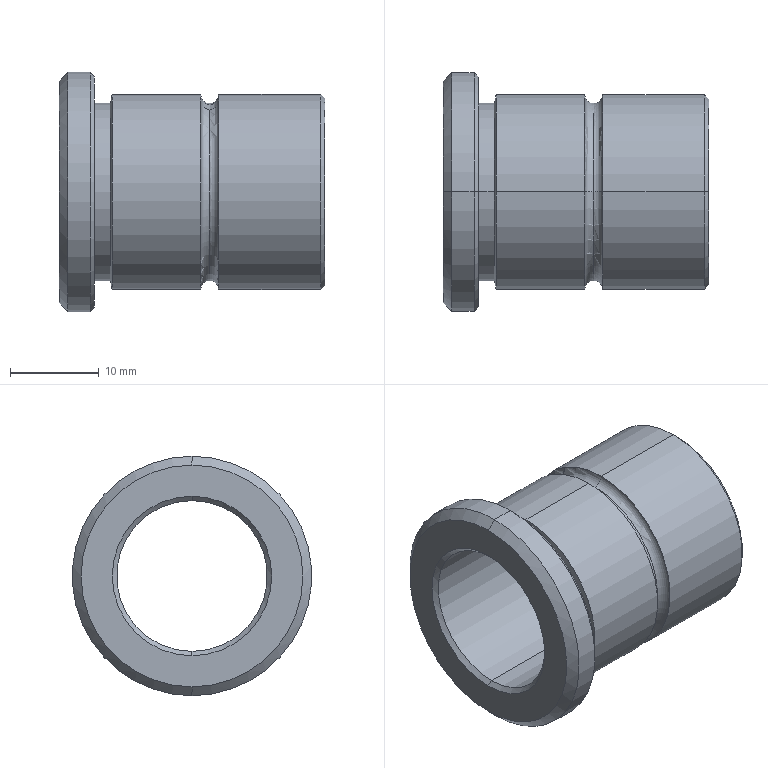Part | SolidWorks | features Chamfer 2, RefAxis 1, RevCut 1, Revolution 1 | 1 solid | 29 faces | box 30 x 27 x 27 mm | volume 5060 mm3 | cone 12 | cylinder 10 | torus 4 | plane 3 | commonest cylinder face diameters 22 x4 17 x2 20 x2 27 x2
STEP:
#1=CARTESIAN_POINT('',(18.,0.,-11.));
#2=VERTEX_POINT('',#1);
#3=CARTESIAN_POINT('',(17.,0.,-10.));
#4=VERTEX_POINT('',#3);
#5=CARTESIAN_POINT('',(17.,0.,-11.));
#6=DIRECTION('',(0.,-1.,0.));
#7=DIRECTION('',(0.,0.,-1.));
#8=AXIS2_PLACEMENT_3D('',#5,#6,#7);
#9=CIRCLE('',#8,1.);
#10=EDGE_CURVE('',#2,#4,#9,.T.);
#11=ORIENTED_EDGE('',*,*,#10,.T.);
#12=CARTESIAN_POINT('',(17.,0.,10.));
#13=VERTEX_POINT('',#12);
#14=CARTESIAN_POINT('',(17.,0.,0.));
#15=DIRECTION('',(1.,0.,0.));
#16=DIRECTION('',(0.,0.,-1.));
#17=AXIS2_PLACEMENT_3D('',#14,#15,#16);
#18=CIRCLE('',#17,10.);
#19=EDGE_CURVE('',#4,#13,#18,.T.);
#20=ORIENTED_EDGE('',*,*,#19,.T.);
#21=CARTESIAN_POINT('',(18.,0.,11.));
#22=VERTEX_POINT('',#21);
#23=CARTESIAN_POINT('',(17.,0.,11.));
#24=DIRECTION('',(0.,1.,0.));
#25=DIRECTION('',(0.,0.,1.));
#26=AXIS2_PLACEMENT_3D('',#23,#24,#25);
#27=CIRCLE('',#26,1.);
#28=EDGE_CURVE('',#22,#13,#27,.T.);
#29=ORIENTED_EDGE('',*,*,#28,.F.);
#30=CARTESIAN_POINT('',(18.,0.,0.));
#31=DIRECTION('',(1.,0.,0.));
#32=DIRECTION('',(0.,0.,1.));
#33=AXIS2_PLACEMENT_3D('',#30,#31,#32);
#34=CIRCLE('',#33,11.);
#35=EDGE_CURVE('',#2,#22,#34,.T.);
#36=ORIENTED_EDGE('',*,*,#35,.F.);
#37=EDGE_LOOP('',(#11,#20,#29,#36));
#38=FACE_OUTER_BOUND('',#37,.T.);
#39=CARTESIAN_POINT('',(17.,0.,0.));
#40=DIRECTION('',(1.,0.,0.));
#41=DIRECTION('',(0.,0.,-1.));
#42=AXIS2_PLACEMENT_3D('',#39,#40,#41);
#43=TOROIDAL_SURFACE('',#42,11.,1.);
#44=ADVANCED_FACE('',(#38),#43,.F.);
#45=ORIENTED_EDGE('',*,*,#28,.T.);
#46=CARTESIAN_POINT('',(17.,0.,0.));
#47=DIRECTION('',(1.,0.,0.));
#48=DIRECTION('',(0.,0.,-1.));
#49=AXIS2_PLACEMENT_3D('',#46,#47,#48);
#50=CIRCLE('',#49,10.);
#51=EDGE_CURVE('',#13,#4,#50,.T.);
#52=ORIENTED_EDGE('',*,*,#51,.T.);
#53=ORIENTED_EDGE('',*,*,#10,.F.);
#54=CARTESIAN_POINT('',(18.,0.,0.));
#55=DIRECTION('',(1.,0.,0.));
#56=DIRECTION('',(0.,0.,1.));
#57=AXIS2_PLACEMENT_3D('',#54,#55,#56);
#58=CIRCLE('',#57,11.);
#59=EDGE_CURVE('',#22,#2,#58,.T.);
#60=ORIENTED_EDGE('',*,*,#59,.F.);
#61=EDGE_LOOP('',(#45,#52,#53,#60));
#62=FACE_OUTER_BOUND('',#61,.T.);
#63=CARTESIAN_POINT('',(17.,0.,0.));
#64=DIRECTION('',(1.,0.,0.));
#65=DIRECTION('',(0.,0.,-1.));
#66=AXIS2_PLACEMENT_3D('',#63,#64,#65);
#67=TOROIDAL_SURFACE('',#66,11.,1.);
#68=ADVANCED_FACE('',(#62),#67,.F.);
#69=CARTESIAN_POINT('',(5.8,0.,-10.));
#70=VERTEX_POINT('',#69);
#71=CARTESIAN_POINT('',(5.8,0.,10.));
#72=VERTEX_POINT('',#71);
#73=CARTESIAN_POINT('',(5.8,0.,0.));
#74=DIRECTION('',(1.,0.,0.));
#75=DIRECTION('',(0.,0.,-1.));
#76=AXIS2_PLACEMENT_3D('',#73,#74,#75);
#77=CIRCLE('',#76,10.);
#78=EDGE_CURVE('',#70,#72,#77,.T.);
#79=ORIENTED_EDGE('',*,*,#78,.T.);
#80=CARTESIAN_POINT('',(6.,0.,11.));
#81=VERTEX_POINT('',#80);
#82=CARTESIAN_POINT('',(5.8,0.,10.));
#83=DIRECTION('',(0.1961,0.,0.9806));
#84=VECTOR('',#83,1000.);
#85=LINE('',#82,#84);
#86=EDGE_CURVE('',#72,#81,#85,.T.);
#87=ORIENTED_EDGE('',*,*,#86,.T.);
#88=CARTESIAN_POINT('',(6.,0.,-11.));
#89=VERTEX_POINT('',#88);
#90=CARTESIAN_POINT('',(6.,0.,0.));
#91=DIRECTION('',(1.,0.,0.));
#92=DIRECTION('',(0.,0.,-1.));
#93=AXIS2_PLACEMENT_3D('',#90,#91,#92);
#94=CIRCLE('',#93,11.);
#95=EDGE_CURVE('',#89,#81,#94,.T.);
#96=ORIENTED_EDGE('',*,*,#95,.F.);
#97=CARTESIAN_POINT('',(5.8,0.,-10.));
#98=DIRECTION('',(0.1961,0.,-0.9806));
#99=VECTOR('',#98,1000.);
#100=LINE('',#97,#99);
#101=EDGE_CURVE('',#70,#89,#100,.T.);
#102=ORIENTED_EDGE('',*,*,#101,.F.);
#103=EDGE_LOOP('',(#79,#87,#96,#102));
#104=FACE_OUTER_BOUND('',#103,.T.);
#105=CARTESIAN_POINT('',(5.8,0.,0.));
#106=DIRECTION('',(1.,0.,0.));
#107=DIRECTION('',(0.,0.,-1.));
#108=AXIS2_PLACEMENT_3D('',#105,#106,#107);
#109=CONICAL_SURFACE('',#108,10.,1.373);
#110=ADVANCED_FACE('',(#104),#109,.T.);
#111=CARTESIAN_POINT('',(4.,0.,-10.));
#112=VERTEX_POINT('',#111);
#113=CARTESIAN_POINT('',(4.,0.,10.));
#114=VERTEX_POINT('',#113);
#115=CARTESIAN_POINT('',(4.,0.,0.));
#116=DIRECTION('',(1.,0.,0.));
#117=DIRECTION('',(0.,0.,-1.));
#118=AXIS2_PLACEMENT_3D('',#115,#116,#117);
#119=CIRCLE('',#118,10.);
#120=EDGE_CURVE('',#112,#114,#119,.T.);
#121=ORIENTED_EDGE('',*,*,#120,.T.);
#122=CARTESIAN_POINT('',(29.5,0.,10.));
#123=DIRECTION('',(1.,0.,0.));
#124=VECTOR('',#123,1000.);
#125=LINE('',#122,#124);
#126=EDGE_CURVE('',#114,#72,#125,.T.);
#127=ORIENTED_EDGE('',*,*,#126,.T.);
#128=ORIENTED_EDGE('',*,*,#78,.F.);
#129=CARTESIAN_POINT('',(29.5,0.,-10.));
#130=DIRECTION('',(1.,0.,0.));
#131=VECTOR('',#130,1000.);
#132=LINE('',#129,#131);
#133=EDGE_CURVE('',#112,#70,#132,.T.);
#134=ORIENTED_EDGE('',*,*,#133,.F.);
#135=EDGE_LOOP('',(#121,#127,#128,#134));
#136=FACE_OUTER_BOUND('',#135,.T.);
#137=CARTESIAN_POINT('',(29.5,0.,0.));
#138=DIRECTION('',(1.,0.,0.));
#139=DIRECTION('',(0.,0.,-1.));
#140=AXIS2_PLACEMENT_3D('',#137,#138,#139);
#141=CYLINDRICAL_SURFACE('',#140,10.);
#142=ADVANCED_FACE('',(#136),#141,.T.);
#143=ORIENTED_EDGE('',*,*,#51,.F.);
#144=CARTESIAN_POINT('',(16.,0.,11.));
#145=VERTEX_POINT('',#144);
#146=CARTESIAN_POINT('',(17.,0.,11.));
#147=DIRECTION('',(0.,1.,0.));
#148=DIRECTION('',(0.,0.,1.));
#149=AXIS2_PLACEMENT_3D('',#146,#147,#148);
#150=CIRCLE('',#149,1.);
#151=EDGE_CURVE('',#13,#145,#150,.T.);
#152=ORIENTED_EDGE('',*,*,#151,.T.);
#153=CARTESIAN_POINT('',(16.,0.,-11.));
#154=VERTEX_POINT('',#153);
#155=CARTESIAN_POINT('',(16.,0.,0.));
#156=DIRECTION('',(-1.,0.,0.));
#157=DIRECTION('',(0.,0.,-1.));
#158=AXIS2_PLACEMENT_3D('',#155,#156,#157);
#159=CIRCLE('',#158,11.);
#160=EDGE_CURVE('',#154,#145,#159,.T.);
#161=ORIENTED_EDGE('',*,*,#160,.F.);
#162=CARTESIAN_POINT('',(17.,0.,-11.));
#163=DIRECTION('',(0.,-1.,0.));
#164=DIRECTION('',(0.,0.,-1.));
#165=AXIS2_PLACEMENT_3D('',#162,#163,#164);
#166=CIRCLE('',#165,1.);
#167=EDGE_CURVE('',#4,#154,#166,.T.);
#168=ORIENTED_EDGE('',*,*,#167,.F.);
#169=EDGE_LOOP('',(#143,#152,#161,#168));
#170=FACE_OUTER_BOUND('',#169,.T.);
#171=CARTESIAN_POINT('',(17.,0.,0.));
#172=DIRECTION('',(1.,0.,0.));
#173=DIRECTION('',(0.,0.,-1.));
#174=AXIS2_PLACEMENT_3D('',#171,#172,#173);
#175=TOROIDAL_SURFACE('',#174,11.,1.);
#176=ADVANCED_FACE('',(#170),#175,.F.);
#177=CARTESIAN_POINT('',(30.,0.,-10.5));
#178=VERTEX_POINT('',#177);
#179=CARTESIAN_POINT('',(30.,0.,10.5));
#180=VERTEX_POINT('',#179);
#181=CARTESIAN_POINT('',(30.,0.,0.));
#182=DIRECTION('',(1.,0.,0.));
#183=DIRECTION('',(0.,0.,1.));
#184=AXIS2_PLACEMENT_3D('',#181,#182,#183);
#185=CIRCLE('',#184,10.5);
#186=EDGE_CURVE('',#178,#180,#185,.T.);
#187=ORIENTED_EDGE('',*,*,#186,.F.);
#188=CARTESIAN_POINT('',(29.5,0.,-11.));
#189=VERTEX_POINT('',#188);
#190=CARTESIAN_POINT('',(29.5,0.,-11.));
#191=DIRECTION('',(-0.7071,0.,-0.7071));
#192=VECTOR('',#191,1000.);
#193=LINE('',#190,#192);
#194=EDGE_CURVE('',#178,#189,#193,.T.);
#195=ORIENTED_EDGE('',*,*,#194,.T.);
#196=CARTESIAN_POINT('',(29.5,0.,11.));
#197=VERTEX_POINT('',#196);
#198=CARTESIAN_POINT('',(29.5,0.,0.));
#199=DIRECTION('',(-1.,0.,0.));
#200=DIRECTION('',(0.,0.,1.));
#201=AXIS2_PLACEMENT_3D('',#198,#199,#200);
#202=CIRCLE('',#201,11.);
#203=EDGE_CURVE('',#197,#189,#202,.T.);
#204=ORIENTED_EDGE('',*,*,#203,.F.);
#205=CARTESIAN_POINT('',(29.5,0.,11.));
#206=DIRECTION('',(-0.7071,0.,0.7071));
#207=VECTOR('',#206,1000.);
#208=LINE('',#205,#207);
#209=EDGE_CURVE('',#180,#197,#208,.T.);
#210=ORIENTED_EDGE('',*,*,#209,.F.);
#211=EDGE_LOOP('',(#187,#195,#204,#210));
#212=FACE_OUTER_BOUND('',#211,.T.);
#213=CARTESIAN_POINT('',(29.5,0.,0.));
#214=DIRECTION('',(-1.,0.,0.));
#215=DIRECTION('',(0.,0.,1.));
#216=AXIS2_PLACEMENT_3D('',#213,#214,#215);
#217=CONICAL_SURFACE('',#216,11.,0.7854);
#218=ADVANCED_FACE('',(#212),#217,.T.);
#219=CARTESIAN_POINT('',(29.5,0.,8.5));
#220=VERTEX_POINT('',#219);
#221=CARTESIAN_POINT('',(29.5,0.,-8.5));
#222=VERTEX_POINT('',#221);
#223=CARTESIAN_POINT('',(29.5,0.,0.));
#224=DIRECTION('',(1.,0.,0.));
#225=DIRECTION('',(0.,0.,1.));
#226=AXIS2_PLACEMENT_3D('',#223,#224,#225);
#227=CIRCLE('',#226,8.5);
#228=EDGE_CURVE('',#220,#222,#227,.T.);
#229=ORIENTED_EDGE('',*,*,#228,.F.);
#230=CARTESIAN_POINT('',(30.,0.,9.));
#231=VERTEX_POINT('',#230);
#232=CARTESIAN_POINT('',(30.,0.,9.));
#233=DIRECTION('',(0.7071,0.,0.7071));
#234=VECTOR('',#233,1000.);
#235=LINE('',#232,#234);
#236=EDGE_CURVE('',#220,#231,#235,.T.);
#237=ORIENTED_EDGE('',*,*,#236,.T.);
#238=CARTESIAN_POINT('',(30.,0.,-9.));
#239=VERTEX_POINT('',#238);
#240=CARTESIAN_POINT('',(30.,0.,0.));
#241=DIRECTION('',(-1.,0.,0.));
#242=DIRECTION('',(0.,0.,1.));
#243=AXIS2_PLACEMENT_3D('',#240,#241,#242);
#244=CIRCLE('',#243,9.);
#245=EDGE_CURVE('',#239,#231,#244,.T.);
#246=ORIENTED_EDGE('',*,*,#245,.F.);
#247=CARTESIAN_POINT('',(30.,0.,-9.));
#248=DIRECTION('',(0.7071,0.,-0.7071));
#249=VECTOR('',#248,1000.);
#250=LINE('',#247,#249);
#251=EDGE_CURVE('',#222,#239,#250,.T.);
#252=ORIENTED_EDGE('',*,*,#251,.F.);
#253=EDGE_LOOP('',(#229,#237,#246,#252));
#254=FACE_OUTER_BOUND('',#253,.T.);
#255=CARTESIAN_POINT('',(30.,0.,0.));
#256=DIRECTION('',(1.,0.,0.));
#257=DIRECTION('',(0.,0.,-1.));
#258=AXIS2_PLACEMENT_3D('',#255,#256,#257);
#259=CONICAL_SURFACE('',#258,9.,0.7854);
#260=ADVANCED_FACE('',(#254),#259,.F.);
#261=CARTESIAN_POINT('',(0.5,0.,-8.5));
#262=VERTEX_POINT('',#261);
#263=CARTESIAN_POINT('',(0.5,0.,8.5));
#264=VERTEX_POINT('',#263);
#265=CARTESIAN_POINT('',(0.5,0.,0.));
#266=DIRECTION('',(-1.,0.,0.));
#267=DIRECTION('',(0.,0.,-1.));
#268=AXIS2_PLACEMENT_3D('',#265,#266,#267);
#269=CIRCLE('',#268,8.5);
#270=EDGE_CURVE('',#262,#264,#269,.T.);
#271=ORIENTED_EDGE('',*,*,#270,.F.);
#272=CARTESIAN_POINT('',(0.,0.,-9.));
#273=VERTEX_POINT('',#272);
#274=CARTESIAN_POINT('',(0.5,0.,-8.5));
#275=DIRECTION('',(-0.7071,0.,-0.7071));
#276=VECTOR('',#275,1000.);
#277=LINE('',#274,#276);
#278=EDGE_CURVE('',#262,#273,#277,.T.);
#279=ORIENTED_EDGE('',*,*,#278,.T.);
#280=CARTESIAN_POINT('',(0.,0.,9.));
#281=VERTEX_POINT('',#280);
#282=CARTESIAN_POINT('',(0.,0.,0.));
#283=DIRECTION('',(1.,0.,0.));
#284=DIRECTION('',(0.,0.,-1.));
#285=AXIS2_PLACEMENT_3D('',#282,#283,#284);
#286=CIRCLE('',#285,9.);
#287=EDGE_CURVE('',#281,#273,#286,.T.);
#288=ORIENTED_EDGE('',*,*,#287,.F.);
#289=CARTESIAN_POINT('',(0.5,0.,8.5));
#290=DIRECTION('',(-0.7071,0.,0.7071));
#291=VECTOR('',#290,1000.);
#292=LINE('',#289,#291);
#293=EDGE_CURVE('',#264,#281,#292,.T.);
#294=ORIENTED_EDGE('',*,*,#293,.F.);
#295=EDGE_LOOP('',(#271,#279,#288,#294));
#296=FACE_OUTER_BOUND('',#295,.T.);
#297=CARTESIAN_POINT('',(0.5,0.,0.));
#298=DIRECTION('',(-1.,0.,0.));
#299=DIRECTION('',(0.,0.,1.));
#300=AXIS2_PLACEMENT_3D('',#297,#298,#299);
#301=CONICAL_SURFACE('',#300,8.5,0.7854);
#302=ADVANCED_FACE('',(#296),#301,.F.);
#303=CARTESIAN_POINT('',(4.,0.,-13.));
#304=VERTEX_POINT('',#303);
#305=CARTESIAN_POINT('',(4.,0.,13.));
#306=VERTEX_POINT('',#305);
#307=CARTESIAN_POINT('',(4.,0.,0.));
#308=DIRECTION('',(1.,0.,0.));
#309=DIRECTION('',(0.,0.,1.));
#310=AXIS2_PLACEMENT_3D('',#307,#308,#309);
#311=CIRCLE('',#310,13.);
#312=EDGE_CURVE('',#304,#306,#311,.T.);
#313=ORIENTED_EDGE('',*,*,#312,.F.);
#314=CARTESIAN_POINT('',(3.5,0.,-13.5));
#315=VERTEX_POINT('',#314);
#316=CARTESIAN_POINT('',(3.5,0.,-13.5));
#317=DIRECTION('',(-0.7071,0.,-0.7071));
#318=VECTOR('',#317,1000.);
#319=LINE('',#316,#318);
#320=EDGE_CURVE('',#304,#315,#319,.T.);
#321=ORIENTED_EDGE('',*,*,#320,.T.);
#322=CARTESIAN_POINT('',(3.5,0.,13.5));
#323=VERTEX_POINT('',#322);
#324=CARTESIAN_POINT('',(3.5,0.,0.));
#325=DIRECTION('',(-1.,0.,0.));
#326=DIRECTION('',(0.,0.,1.));
#327=AXIS2_PLACEMENT_3D('',#324,#325,#326);
#328=CIRCLE('',#327,13.5);
#329=EDGE_CURVE('',#323,#315,#328,.T.);
#330=ORIENTED_EDGE('',*,*,#329,.F.);
#331=CARTESIAN_POINT('',(3.5,0.,13.5));
#332=DIRECTION('',(-0.7071,0.,0.7071));
#333=VECTOR('',#332,1000.);
#334=LINE('',#331,#333);
#335=EDGE_CURVE('',#306,#323,#334,.T.);
#336=ORIENTED_EDGE('',*,*,#335,.F.);
#337=EDGE_LOOP('',(#313,#321,#330,#336));
#338=FACE_OUTER_BOUND('',#337,.T.);
#339=CARTESIAN_POINT('',(3.5,0.,0.));
#340=DIRECTION('',(-1.,0.,0.));
#341=DIRECTION('',(0.,0.,1.));
#342=AXIS2_PLACEMENT_3D('',#339,#340,#341);
#343=CONICAL_SURFACE('',#342,13.5,0.7854);
#344=ADVANCED_FACE('',(#338),#343,.T.);
#345=CARTESIAN_POINT('',(0.,0.,12.5));
#346=VERTEX_POINT('',#345);
#347=CARTESIAN_POINT('',(0.,0.,-12.5));
#348=VERTEX_POINT('',#347);
#349=CARTESIAN_POINT('',(0.,0.,0.));
#350=DIRECTION('',(-1.,0.,0.));
#351=DIRECTION('',(0.,0.,-1.));
#352=AXIS2_PLACEMENT_3D('',#349,#350,#351);
#353=CIRCLE('',#352,12.5);
#354=EDGE_CURVE('',#346,#348,#353,.T.);
#355=ORIENTED_EDGE('',*,*,#354,.F.);
#356=CARTESIAN_POINT('',(1.,0.,13.5));
#357=VERTEX_POINT('',#356);
#358=CARTESIAN_POINT('',(0.,0.,12.5));
#359=DIRECTION('',(0.7071,0.,0.7071));
#360=VECTOR('',#359,1000.);
#361=LINE('',#358,#360);
#362=EDGE_CURVE('',#346,#357,#361,.T.);
#363=ORIENTED_EDGE('',*,*,#362,.T.);
#364=CARTESIAN_POINT('',(1.,0.,-13.5));
#365=VERTEX_POINT('',#364);
#366=CARTESIAN_POINT('',(1.,0.,0.));
#367=DIRECTION('',(1.,0.,0.));
#368=DIRECTION('',(0.,0.,-1.));
#369=AXIS2_PLACEMENT_3D('',#366,#367,#368);
#370=CIRCLE('',#369,13.5);
#371=EDGE_CURVE('',#365,#357,#370,.T.);
#372=ORIENTED_EDGE('',*,*,#371,.F.);
#373=CARTESIAN_POINT('',(0.,0.,-12.5));
#374=DIRECTION('',(0.7071,0.,-0.7071));
#375=VECTOR('',#374,1000.);
#376=LINE('',#373,#375);
#377=EDGE_CURVE('',#348,#365,#376,.T.);
#378=ORIENTED_EDGE('',*,*,#377,.F.);
#379=EDGE_LOOP('',(#355,#363,#372,#378));
#380=FACE_OUTER_BOUND('',#379,.T.);
#381=CARTESIAN_POINT('',(0.,0.,0.));
#382=DIRECTION('',(1.,0.,0.));
#383=DIRECTION('',(0.,0.,-1.));
#384=AXIS2_PLACEMENT_3D('',#381,#382,#383);
#385=CONICAL_SURFACE('',#384,12.5,0.7854);
#386=ADVANCED_FACE('',(#380),#385,.T.);
#387=CARTESIAN_POINT('',(16.,0.,0.));
#388=DIRECTION('',(-1.,0.,0.));
#389=DIRECTION('',(0.,0.,-1.));
#390=AXIS2_PLACEMENT_3D('',#387,#388,#389);
#391=CIRCLE('',#390,11.);
#392=EDGE_CURVE('',#145,#154,#391,.T.);
#393=ORIENTED_EDGE('',*,*,#392,.T.);
#394=CARTESIAN_POINT('',(0.,0.,-11.));
#395=DIRECTION('',(-1.,0.,0.));
#396=VECTOR('',#395,1000.);
#397=LINE('',#394,#396);
#398=EDGE_CURVE('',#154,#89,#397,.T.);
#399=ORIENTED_EDGE('',*,*,#398,.T.);
#400=ORIENTED_EDGE('',*,*,#95,.T.);
#401=CARTESIAN_POINT('',(0.,0.,11.));
#402=DIRECTION('',(-1.,0.,0.));
#403=VECTOR('',#402,1000.);
#404=LINE('',#401,#403);
#405=EDGE_CURVE('',#145,#81,#404,.T.);
#406=ORIENTED_EDGE('',*,*,#405,.F.);
#407=EDGE_LOOP('',(#393,#399,#400,#406));
#408=FACE_OUTER_BOUND('',#407,.T.);
#409=CARTESIAN_POINT('',(0.,0.,0.));
#410=DIRECTION('',(-1.,0.,0.));
#411=DIRECTION('',(0.,0.,1.));
#412=AXIS2_PLACEMENT_3D('',#409,#410,#411);
#413=CYLINDRICAL_SURFACE('',#412,11.);
#414=ADVANCED_FACE('',(#408),#413,.T.);
#415=ORIENTED_EDGE('',*,*,#329,.T.);
#416=CARTESIAN_POINT('',(0.,0.,-13.5));
#417=DIRECTION('',(-1.,0.,0.));
#418=VECTOR('',#417,1000.);
#419=LINE('',#416,#418);
#420=EDGE_CURVE('',#315,#365,#419,.T.);
#421=ORIENTED_EDGE('',*,*,#420,.T.);
#422=ORIENTED_EDGE('',*,*,#371,.T.);
#423=CARTESIAN_POINT('',(0.,0.,13.5));
#424=DIRECTION('',(-1.,0.,0.));
#425=VECTOR('',#424,1000.);
#426=LINE('',#423,#425);
#427=EDGE_CURVE('',#323,#357,#426,.T.);
#428=ORIENTED_EDGE('',*,*,#427,.F.);
#429=EDGE_LOOP('',(#415,#421,#422,#428));
#430=FACE_OUTER_BOUND('',#429,.T.);
#431=CARTESIAN_POINT('',(0.,0.,0.));
#432=DIRECTION('',(-1.,0.,0.));
#433=DIRECTION('',(0.,0.,1.));
#434=AXIS2_PLACEMENT_3D('',#431,#432,#433);
#435=CYLINDRICAL_SURFACE('',#434,13.5);
#436=ADVANCED_FACE('',(#430),#435,.T.);
#437=ORIENTED_EDGE('',*,*,#228,.T.);
#438=CARTESIAN_POINT('',(0.,0.,-8.5));
#439=DIRECTION('',(-1.,0.,0.));
#440=VECTOR('',#439,1000.);
#441=LINE('',#438,#440);
#442=EDGE_CURVE('',#222,#262,#441,.T.);
#443=ORIENTED_EDGE('',*,*,#442,.T.);
#444=ORIENTED_EDGE('',*,*,#270,.T.);
#445=CARTESIAN_POINT('',(0.,0.,8.5));
#446=DIRECTION('',(-1.,0.,0.));
#447=VECTOR('',#446,1000.);
#448=LINE('',#445,#447);
#449=EDGE_CURVE('',#220,#264,#448,.T.);
#450=ORIENTED_EDGE('',*,*,#449,.F.);
#451=EDGE_LOOP('',(#437,#443,#444,#450));
#452=FACE_OUTER_BOUND('',#451,.T.);
#453=CARTESIAN_POINT('',(0.,0.,0.));
#454=DIRECTION('',(-1.,0.,0.));
#455=DIRECTION('',(0.,0.,1.));
#456=AXIS2_PLACEMENT_3D('',#453,#454,#455);
#457=CYLINDRICAL_SURFACE('',#456,8.5);
#458=ADVANCED_FACE('',(#452),#457,.F.);
#459=ORIENTED_EDGE('',*,*,#203,.T.);
#460=CARTESIAN_POINT('',(0.,0.,-11.));
#461=DIRECTION('',(-1.,0.,0.));
#462=VECTOR('',#461,1000.);
#463=LINE('',#460,#462);
#464=EDGE_CURVE('',#189,#2,#463,.T.);
#465=ORIENTED_EDGE('',*,*,#464,.T.);
#466=ORIENTED_EDGE('',*,*,#35,.T.);
#467=CARTESIAN_POINT('',(0.,0.,11.));
#468=DIRECTION('',(-1.,0.,0.));
#469=VECTOR('',#468,1000.);
#470=LINE('',#467,#469);
#471=EDGE_CURVE('',#197,#22,#470,.T.);
#472=ORIENTED_EDGE('',*,*,#471,.F.);
#473=EDGE_LOOP('',(#459,#465,#466,#472));
#474=FACE_OUTER_BOUND('',#473,.T.);
#475=CARTESIAN_POINT('',(0.,0.,0.));
#476=DIRECTION('',(-1.,0.,0.));
#477=DIRECTION('',(0.,0.,1.));
#478=AXIS2_PLACEMENT_3D('',#475,#476,#477);
#479=CYLINDRICAL_SURFACE('',#478,11.);
#480=ADVANCED_FACE('',(#474),#479,.T.);
#481=ORIENTED_EDGE('',*,*,#464,.F.);
#482=CARTESIAN_POINT('',(29.5,0.,0.));
#483=DIRECTION('',(-1.,0.,0.));
#484=DIRECTION('',(0.,0.,1.));
#485=AXIS2_PLACEMENT_3D('',#482,#483,#484);
#486=CIRCLE('',#485,11.);
#487=EDGE_CURVE('',#189,#197,#486,.T.);
#488=ORIENTED_EDGE('',*,*,#487,.T.);
#489=ORIENTED_EDGE('',*,*,#471,.T.);
#490=ORIENTED_EDGE('',*,*,#59,.T.);
#491=EDGE_LOOP('',(#481,#488,#489,#490));
#492=FACE_OUTER_BOUND('',#491,.T.);
#493=CARTESIAN_POINT('',(0.,0.,0.));
#494=DIRECTION('',(-1.,0.,0.));
#495=DIRECTION('',(0.,0.,1.));
#496=AXIS2_PLACEMENT_3D('',#493,#494,#495);
#497=CYLINDRICAL_SURFACE('',#496,11.);
#498=ADVANCED_FACE('',(#492),#497,.T.);
#499=ORIENTED_EDGE('',*,*,#245,.T.);
#500=CARTESIAN_POINT('',(30.,0.,0.));
#501=DIRECTION('',(-1.,0.,0.));
#502=DIRECTION('',(0.,0.,1.));
#503=AXIS2_PLACEMENT_3D('',#500,#501,#502);
#504=CIRCLE('',#503,9.);
#505=EDGE_CURVE('',#231,#239,#504,.T.);
#506=ORIENTED_EDGE('',*,*,#505,.T.);
#507=EDGE_LOOP('',(#499,#506));
#508=FACE_BOUND('',#507,.T.);
#509=CARTESIAN_POINT('',(30.,0.,0.));
#510=DIRECTION('',(1.,0.,0.));
#511=DIRECTION('',(0.,0.,1.));
#512=AXIS2_PLACEMENT_3D('',#509,#510,#511);
#513=CIRCLE('',#512,10.5);
#514=EDGE_CURVE('',#180,#178,#513,.T.);
#515=ORIENTED_EDGE('',*,*,#514,.T.);
#516=ORIENTED_EDGE('',*,*,#186,.T.);
#517=EDGE_LOOP('',(#515,#516));
#518=FACE_OUTER_BOUND('',#517,.T.);
#519=CARTESIAN_POINT('',(30.,11.,0.));
#520=DIRECTION('',(-1.,0.,0.));
#521=DIRECTION('',(0.,0.,1.));
#522=AXIS2_PLACEMENT_3D('',#519,#520,#521);
#523=PLANE('',#522);
#524=ADVANCED_FACE('',(#508,#518),#523,.F.);
#525=ORIENTED_EDGE('',*,*,#442,.F.);
#526=CARTESIAN_POINT('',(29.5,0.,0.));
#527=DIRECTION('',(1.,0.,0.));
#528=DIRECTION('',(0.,0.,1.));
#529=AXIS2_PLACEMENT_3D('',#526,#527,#528);
#530=CIRCLE('',#529,8.5);
#531=EDGE_CURVE('',#222,#220,#530,.T.);
#532=ORIENTED_EDGE('',*,*,#531,.T.);
#533=ORIENTED_EDGE('',*,*,#449,.T.);
#534=CARTESIAN_POINT('',(0.5,0.,0.));
#535=DIRECTION('',(-1.,0.,0.));
#536=DIRECTION('',(0.,0.,-1.));
#537=AXIS2_PLACEMENT_3D('',#534,#535,#536);
#538=CIRCLE('',#537,8.5);
#539=EDGE_CURVE('',#264,#262,#538,.T.);
#540=ORIENTED_EDGE('',*,*,#539,.T.);
#541=EDGE_LOOP('',(#525,#532,#533,#540));
#542=FACE_OUTER_BOUND('',#541,.T.);
#543=CARTESIAN_POINT('',(0.,0.,0.));
#544=DIRECTION('',(-1.,0.,0.));
#545=DIRECTION('',(0.,0.,1.));
#546=AXIS2_PLACEMENT_3D('',#543,#544,#545);
#547=CYLINDRICAL_SURFACE('',#546,8.5);
#548=ADVANCED_FACE('',(#542),#547,.F.);
#549=ORIENTED_EDGE('',*,*,#287,.T.);
#550=CARTESIAN_POINT('',(0.,0.,0.));
#551=DIRECTION('',(1.,0.,0.));
#552=DIRECTION('',(0.,0.,-1.));
#553=AXIS2_PLACEMENT_3D('',#550,#551,#552);
#554=CIRCLE('',#553,9.);
#555=EDGE_CURVE('',#273,#281,#554,.T.);
#556=ORIENTED_EDGE('',*,*,#555,.T.);
#557=EDGE_LOOP('',(#549,#556));
#558=FACE_BOUND('',#557,.T.);
#559=CARTESIAN_POINT('',(0.,0.,0.));
#560=DIRECTION('',(-1.,0.,0.));
#561=DIRECTION('',(0.,0.,-1.));
#562=AXIS2_PLACEMENT_3D('',#559,#560,#561);
#563=CIRCLE('',#562,12.5);
#564=EDGE_CURVE('',#348,#346,#563,.T.);
#565=ORIENTED_EDGE('',*,*,#564,.T.);
#566=ORIENTED_EDGE('',*,*,#354,.T.);
#567=EDGE_LOOP('',(#565,#566));
#568=FACE_OUTER_BOUND('',#567,.T.);
#569=CARTESIAN_POINT('',(0.,8.5,0.));
#570=DIRECTION('',(1.,0.,0.));
#571=DIRECTION('',(0.,0.,-1.));
#572=AXIS2_PLACEMENT_3D('',#569,#570,#571);
#573=PLANE('',#572);
#574=ADVANCED_FACE('',(#558,#568),#573,.F.);
#575=ORIENTED_EDGE('',*,*,#420,.F.);
#576=CARTESIAN_POINT('',(3.5,0.,0.));
#577=DIRECTION('',(-1.,0.,0.));
#578=DIRECTION('',(0.,0.,1.));
#579=AXIS2_PLACEMENT_3D('',#576,#577,#578);
#580=CIRCLE('',#579,13.5);
#581=EDGE_CURVE('',#315,#323,#580,.T.);
#582=ORIENTED_EDGE('',*,*,#581,.T.);
#583=ORIENTED_EDGE('',*,*,#427,.T.);
#584=CARTESIAN_POINT('',(1.,0.,0.));
#585=DIRECTION('',(1.,0.,0.));
#586=DIRECTION('',(0.,0.,-1.));
#587=AXIS2_PLACEMENT_3D('',#584,#585,#586);
#588=CIRCLE('',#587,13.5);
#589=EDGE_CURVE('',#357,#365,#588,.T.);
#590=ORIENTED_EDGE('',*,*,#589,.T.);
#591=EDGE_LOOP('',(#575,#582,#583,#590));
#592=FACE_OUTER_BOUND('',#591,.T.);
#593=CARTESIAN_POINT('',(0.,0.,0.));
#594=DIRECTION('',(-1.,0.,0.));
#595=DIRECTION('',(0.,0.,1.));
#596=AXIS2_PLACEMENT_3D('',#593,#594,#595);
#597=CYLINDRICAL_SURFACE('',#596,13.5);
#598=ADVANCED_FACE('',(#592),#597,.T.);
#599=CARTESIAN_POINT('',(4.,0.,0.));
#600=DIRECTION('',(1.,0.,0.));
#601=DIRECTION('',(0.,0.,1.));
#602=AXIS2_PLACEMENT_3D('',#599,#600,#601);
#603=CIRCLE('',#602,13.);
#604=EDGE_CURVE('',#306,#304,#603,.T.);
#605=ORIENTED_EDGE('',*,*,#604,.T.);
#606=ORIENTED_EDGE('',*,*,#312,.T.);
#607=EDGE_LOOP('',(#605,#606));
#608=FACE_OUTER_BOUND('',#607,.T.);
#609=ORIENTED_EDGE('',*,*,#120,.F.);
#610=CARTESIAN_POINT('',(4.,0.,0.));
#611=DIRECTION('',(1.,0.,0.));
#612=DIRECTION('',(0.,0.,-1.));
#613=AXIS2_PLACEMENT_3D('',#610,#611,#612);
#614=CIRCLE('',#613,10.);
#615=EDGE_CURVE('',#114,#112,#614,.T.);
#616=ORIENTED_EDGE('',*,*,#615,.F.);
#617=EDGE_LOOP('',(#609,#616));
#618=FACE_BOUND('',#617,.T.);
#619=CARTESIAN_POINT('',(4.,13.5,0.));
#620=DIRECTION('',(-1.,0.,0.));
#621=DIRECTION('',(0.,0.,1.));
#622=AXIS2_PLACEMENT_3D('',#619,#620,#621);
#623=PLANE('',#622);
#624=ADVANCED_FACE('',(#608,#618),#623,.F.);
#625=ORIENTED_EDGE('',*,*,#398,.F.);
#626=ORIENTED_EDGE('',*,*,#160,.T.);
#627=ORIENTED_EDGE('',*,*,#405,.T.);
#628=CARTESIAN_POINT('',(6.,0.,0.));
#629=DIRECTION('',(1.,0.,0.));
#630=DIRECTION('',(0.,0.,-1.));
#631=AXIS2_PLACEMENT_3D('',#628,#629,#630);
#632=CIRCLE('',#631,11.);
#633=EDGE_CURVE('',#81,#89,#632,.T.);
#634=ORIENTED_EDGE('',*,*,#633,.T.);
#635=EDGE_LOOP('',(#625,#626,#627,#634));
#636=FACE_OUTER_BOUND('',#635,.T.);
#637=CARTESIAN_POINT('',(0.,0.,0.));
#638=DIRECTION('',(-1.,0.,0.));
#639=DIRECTION('',(0.,0.,1.));
#640=AXIS2_PLACEMENT_3D('',#637,#638,#639);
#641=CYLINDRICAL_SURFACE('',#640,11.);
#642=ADVANCED_FACE('',(#636),#641,.T.);
#643=ORIENTED_EDGE('',*,*,#362,.F.);
#644=ORIENTED_EDGE('',*,*,#564,.F.);
#645=ORIENTED_EDGE('',*,*,#377,.T.);
#646=ORIENTED_EDGE('',*,*,#589,.F.);
#647=EDGE_LOOP('',(#643,#644,#645,#646));
#648=FACE_OUTER_BOUND('',#647,.T.);
#649=CARTESIAN_POINT('',(0.,0.,0.));
#650=DIRECTION('',(1.,0.,0.));
#651=DIRECTION('',(0.,0.,-1.));
#652=AXIS2_PLACEMENT_3D('',#649,#650,#651);
#653=CONICAL_SURFACE('',#652,12.5,0.7854);
#654=ADVANCED_FACE('',(#648),#653,.T.);
#655=ORIENTED_EDGE('',*,*,#320,.F.);
#656=ORIENTED_EDGE('',*,*,#604,.F.);
#657=ORIENTED_EDGE('',*,*,#335,.T.);
#658=ORIENTED_EDGE('',*,*,#581,.F.);
#659=EDGE_LOOP('',(#655,#656,#657,#658));
#660=FACE_OUTER_BOUND('',#659,.T.);
#661=CARTESIAN_POINT('',(3.5,0.,0.));
#662=DIRECTION('',(-1.,0.,0.));
#663=DIRECTION('',(0.,0.,1.));
#664=AXIS2_PLACEMENT_3D('',#661,#662,#663);
#665=CONICAL_SURFACE('',#664,13.5,0.7854);
#666=ADVANCED_FACE('',(#660),#665,.T.);
#667=ORIENTED_EDGE('',*,*,#278,.F.);
#668=ORIENTED_EDGE('',*,*,#539,.F.);
#669=ORIENTED_EDGE('',*,*,#293,.T.);
#670=ORIENTED_EDGE('',*,*,#555,.F.);
#671=EDGE_LOOP('',(#667,#668,#669,#670));
#672=FACE_OUTER_BOUND('',#671,.T.);
#673=CARTESIAN_POINT('',(0.5,0.,0.));
#674=DIRECTION('',(-1.,0.,0.));
#675=DIRECTION('',(0.,0.,1.));
#676=AXIS2_PLACEMENT_3D('',#673,#674,#675);
#677=CONICAL_SURFACE('',#676,8.5,0.7854);
#678=ADVANCED_FACE('',(#672),#677,.F.);
#679=ORIENTED_EDGE('',*,*,#236,.F.);
#680=ORIENTED_EDGE('',*,*,#531,.F.);
#681=ORIENTED_EDGE('',*,*,#251,.T.);
#682=ORIENTED_EDGE('',*,*,#505,.F.);
#683=EDGE_LOOP('',(#679,#680,#681,#682));
#684=FACE_OUTER_BOUND('',#683,.T.);
#685=CARTESIAN_POINT('',(30.,0.,0.));
#686=DIRECTION('',(1.,0.,0.));
#687=DIRECTION('',(0.,0.,-1.));
#688=AXIS2_PLACEMENT_3D('',#685,#686,#687);
#689=CONICAL_SURFACE('',#688,9.,0.7854);
#690=ADVANCED_FACE('',(#684),#689,.F.);
#691=ORIENTED_EDGE('',*,*,#194,.F.);
#692=ORIENTED_EDGE('',*,*,#514,.F.);
#693=ORIENTED_EDGE('',*,*,#209,.T.);
#694=ORIENTED_EDGE('',*,*,#487,.F.);
#695=EDGE_LOOP('',(#691,#692,#693,#694));
#696=FACE_OUTER_BOUND('',#695,.T.);
#697=CARTESIAN_POINT('',(29.5,0.,0.));
#698=DIRECTION('',(-1.,0.,0.));
#699=DIRECTION('',(0.,0.,1.));
#700=AXIS2_PLACEMENT_3D('',#697,#698,#699);
#701=CONICAL_SURFACE('',#700,11.,0.7854);
#702=ADVANCED_FACE('',(#696),#701,.T.);
#703=ORIENTED_EDGE('',*,*,#19,.F.);
#704=ORIENTED_EDGE('',*,*,#167,.T.);
#705=ORIENTED_EDGE('',*,*,#392,.F.);
#706=ORIENTED_EDGE('',*,*,#151,.F.);
#707=EDGE_LOOP('',(#703,#704,#705,#706));
#708=FACE_OUTER_BOUND('',#707,.T.);
#709=CARTESIAN_POINT('',(17.,0.,0.));
#710=DIRECTION('',(1.,0.,0.));
#711=DIRECTION('',(0.,0.,-1.));
#712=AXIS2_PLACEMENT_3D('',#709,#710,#711);
#713=TOROIDAL_SURFACE('',#712,11.,1.);
#714=ADVANCED_FACE('',(#708),#713,.F.);
#715=ORIENTED_EDGE('',*,*,#126,.F.);
#716=ORIENTED_EDGE('',*,*,#615,.T.);
#717=ORIENTED_EDGE('',*,*,#133,.T.);
#718=CARTESIAN_POINT('',(5.8,0.,0.));
#719=DIRECTION('',(1.,0.,0.));
#720=DIRECTION('',(0.,0.,-1.));
#721=AXIS2_PLACEMENT_3D('',#718,#719,#720);
#722=CIRCLE('',#721,10.);
#723=EDGE_CURVE('',#72,#70,#722,.T.);
#724=ORIENTED_EDGE('',*,*,#723,.F.);
#725=EDGE_LOOP('',(#715,#716,#717,#724));
#726=FACE_OUTER_BOUND('',#725,.T.);
#727=CARTESIAN_POINT('',(29.5,0.,0.));
#728=DIRECTION('',(1.,0.,0.));
#729=DIRECTION('',(0.,0.,-1.));
#730=AXIS2_PLACEMENT_3D('',#727,#728,#729);
#731=CYLINDRICAL_SURFACE('',#730,10.);
#732=ADVANCED_FACE('',(#726),#731,.T.);
#733=ORIENTED_EDGE('',*,*,#86,.F.);
#734=ORIENTED_EDGE('',*,*,#723,.T.);
#735=ORIENTED_EDGE('',*,*,#101,.T.);
#736=ORIENTED_EDGE('',*,*,#633,.F.);
#737=EDGE_LOOP('',(#733,#734,#735,#736));
#738=FACE_OUTER_BOUND('',#737,.T.);
#739=CARTESIAN_POINT('',(5.8,0.,0.));
#740=DIRECTION('',(1.,0.,0.));
#741=DIRECTION('',(0.,0.,-1.));
#742=AXIS2_PLACEMENT_3D('',#739,#740,#741);
#743=CONICAL_SURFACE('',#742,10.,1.373);
#744=ADVANCED_FACE('',(#738),#743,.T.);
#745=CLOSED_SHELL('',(#44,#68,#110,#142,#176,#218,#260,#302,#344,#386,#414,#436,#458,#480,#498,#524,#548,#574,#598,#624,#642,#654,#666,#678,#690,#702,#714,#732,#744));
#746=MANIFOLD_SOLID_BREP('',#745);
#747=CARTESIAN_POINT('',(0.,0.,0.));
#748=DIRECTION('',(0.,0.,1.));
#749=DIRECTION('',(1.,0.,0.));
#750=AXIS2_PLACEMENT_3D('',#747,#748,#749);
#751=(LENGTH_UNIT()NAMED_UNIT(*)SI_UNIT(.MILLI.,.METRE.));
#752=UNCERTAINTY_MEASURE_WITH_UNIT(LENGTH_MEASURE(0.00001),#751,'','');
#753=(NAMED_UNIT(*)PLANE_ANGLE_UNIT()SI_UNIT($,.RADIAN.));
#754=(NAMED_UNIT(*)SI_UNIT($,.STERADIAN.)SOLID_ANGLE_UNIT());
#755=(GEOMETRIC_REPRESENTATION_CONTEXT(3)GLOBAL_UNCERTAINTY_ASSIGNED_CONTEXT((#752))GLOBAL_UNIT_ASSIGNED_CONTEXT((#751,#753,#754))REPRESENTATION_CONTEXT('',''));
#756=ADVANCED_BREP_SHAPE_REPRESENTATION('',(#746,#750),#755);